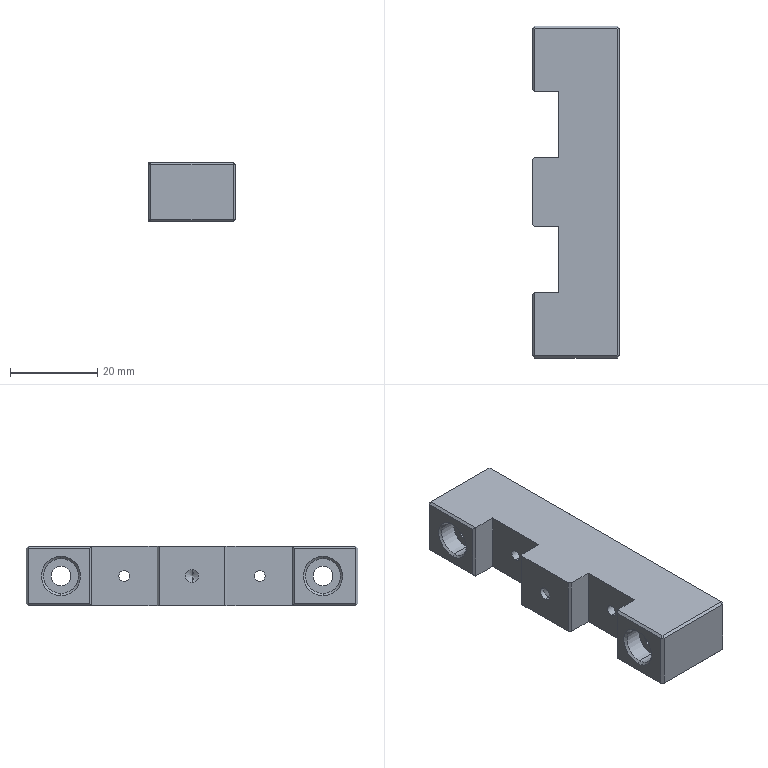Part | SolidWorks | features HoleWzd 4, Chamfer 2, Extrusion 1, ICE 1 | 1 solid | 82 faces | box 20 x 76 x 13.6 mm | volume 16812 mm3 | plane 42 | cone 22 | cylinder 18 | commonest cylinder face diameters 2.5 x4 4 x4 4.5 x4 8 x4 3 x2